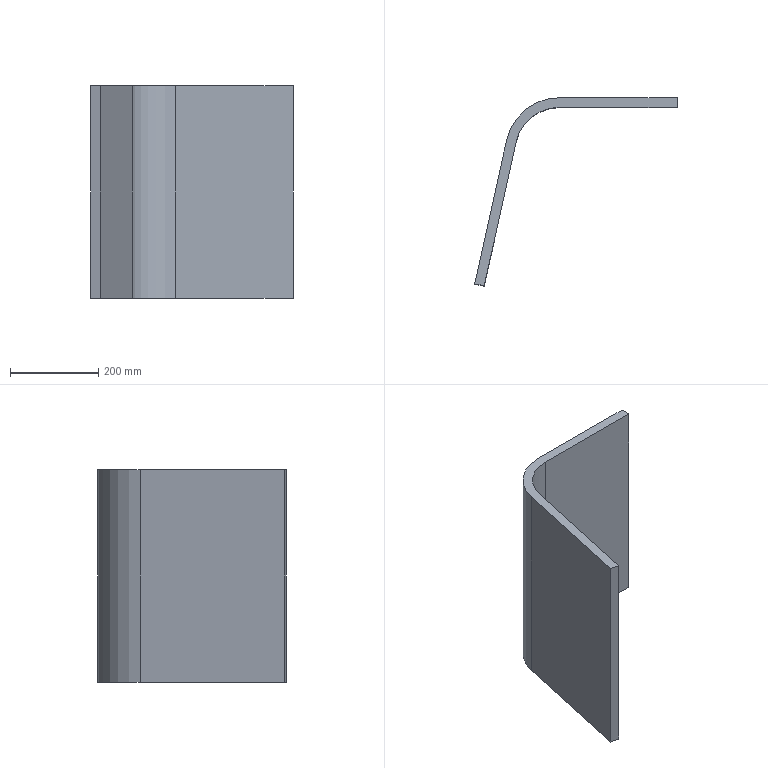Part | NX | features 底座(默认<按焊接>) 2 | 1 solid | 10 faces | box 457.703 x 425.5 x 480 mm | volume 7854055 mm3 | plane 8 | cylinder 2 | commonest cylinder face diameters 200 x1 243.64 x1
STEP:
#1=CARTESIAN_POINT('',(1554.365,567.32,-412.));
#2=VERTEX_POINT('',#1);
#3=CARTESIAN_POINT('',(1287.717,567.32,-412.));
#4=VERTEX_POINT('',#3);
#5=CARTESIAN_POINT('',(1250.85,567.32,-412.));
#6=DIRECTION('',(-1.,0.,0.));
#7=VECTOR('',#6,1000.);
#8=LINE('',#5,#7);
#9=EDGE_CURVE('',#2,#4,#8,.T.);
#10=ORIENTED_EDGE('',*,*,#9,.F.);
#11=CARTESIAN_POINT('',(1554.365,567.32,-892.));
#12=VERTEX_POINT('',#11);
#13=CARTESIAN_POINT('',(1554.365,567.32,-892.));
#14=DIRECTION('',(0.,0.,1.));
#15=VECTOR('',#14,1000.);
#16=LINE('',#13,#15);
#17=EDGE_CURVE('',#12,#2,#16,.T.);
#18=ORIENTED_EDGE('',*,*,#17,.F.);
#19=CARTESIAN_POINT('',(1287.717,567.32,-892.));
#20=VERTEX_POINT('',#19);
#21=CARTESIAN_POINT('',(1250.85,567.32,-892.));
#22=DIRECTION('',(-1.,0.,0.));
#23=VECTOR('',#22,1000.);
#24=LINE('',#21,#23);
#25=EDGE_CURVE('',#12,#20,#24,.T.);
#26=ORIENTED_EDGE('',*,*,#25,.T.);
#27=CARTESIAN_POINT('',(1287.717,567.32,-892.));
#28=DIRECTION('',(0.,0.,1.));
#29=VECTOR('',#28,1000.);
#30=LINE('',#27,#29);
#31=EDGE_CURVE('',#20,#4,#30,.T.);
#32=ORIENTED_EDGE('',*,*,#31,.T.);
#33=EDGE_LOOP('',(#10,#18,#26,#32));
#34=FACE_BOUND('',#33,.T.);
#35=CARTESIAN_POINT('',(1250.85,567.32,-892.));
#36=DIRECTION('',(0.,-1.,0.));
#37=DIRECTION('',(0.,0.,1.));
#38=AXIS2_PLACEMENT_3D('',#35,#36,#37);
#39=PLANE('',#38);
#40=ADVANCED_FACE('',(#34),#39,.F.);
#41=CARTESIAN_POINT('',(1168.785,471.867,-412.));
#42=VERTEX_POINT('',#41);
#43=CARTESIAN_POINT('',(1287.717,445.5,-412.));
#44=DIRECTION('',(0.,0.,1.));
#45=DIRECTION('',(1.,0.,0.));
#46=AXIS2_PLACEMENT_3D('',#43,#44,#45);
#47=CIRCLE('',#46,121.82);
#48=EDGE_CURVE('',#4,#42,#47,.T.);
#49=ORIENTED_EDGE('',*,*,#48,.F.);
#50=ORIENTED_EDGE('',*,*,#31,.F.);
#51=CARTESIAN_POINT('',(1168.785,471.867,-892.));
#52=VERTEX_POINT('',#51);
#53=CARTESIAN_POINT('',(1287.717,445.5,-892.));
#54=DIRECTION('',(0.,0.,1.));
#55=DIRECTION('',(1.,0.,0.));
#56=AXIS2_PLACEMENT_3D('',#53,#54,#55);
#57=CIRCLE('',#56,121.82);
#58=EDGE_CURVE('',#20,#52,#57,.T.);
#59=ORIENTED_EDGE('',*,*,#58,.T.);
#60=CARTESIAN_POINT('',(1168.785,471.867,-892.));
#61=DIRECTION('',(0.,0.,1.));
#62=VECTOR('',#61,1000.);
#63=LINE('',#60,#62);
#64=EDGE_CURVE('',#52,#42,#63,.T.);
#65=ORIENTED_EDGE('',*,*,#64,.T.);
#66=EDGE_LOOP('',(#49,#50,#59,#65));
#67=FACE_BOUND('',#66,.T.);
#68=CARTESIAN_POINT('',(1287.717,445.5,-892.));
#69=DIRECTION('',(0.,0.,1.));
#70=DIRECTION('',(-1.,0.,0.));
#71=AXIS2_PLACEMENT_3D('',#68,#69,#70);
#72=CYLINDRICAL_SURFACE('',#71,121.82);
#73=ADVANCED_FACE('',(#67),#72,.T.);
#74=CARTESIAN_POINT('',(1096.662,146.543,-412.));
#75=VERTEX_POINT('',#74);
#76=CARTESIAN_POINT('',(571.37,-2222.899,-412.));
#77=DIRECTION('',(0.2164,0.9763,0.));
#78=VECTOR('',#77,1000.);
#79=LINE('',#76,#78);
#80=EDGE_CURVE('',#75,#42,#79,.T.);
#81=ORIENTED_EDGE('',*,*,#80,.T.);
#82=ORIENTED_EDGE('',*,*,#64,.F.);
#83=CARTESIAN_POINT('',(1096.662,146.543,-892.));
#84=VERTEX_POINT('',#83);
#85=CARTESIAN_POINT('',(571.37,-2222.899,-892.));
#86=DIRECTION('',(0.2164,0.9763,0.));
#87=VECTOR('',#86,1000.);
#88=LINE('',#85,#87);
#89=EDGE_CURVE('',#84,#52,#88,.T.);
#90=ORIENTED_EDGE('',*,*,#89,.F.);
#91=CARTESIAN_POINT('',(1096.662,146.543,-892.));
#92=DIRECTION('',(0.,0.,1.));
#93=VECTOR('',#92,1000.);
#94=LINE('',#91,#93);
#95=EDGE_CURVE('',#84,#75,#94,.T.);
#96=ORIENTED_EDGE('',*,*,#95,.T.);
#97=EDGE_LOOP('',(#81,#82,#90,#96));
#98=FACE_BOUND('',#97,.T.);
#99=CARTESIAN_POINT('',(571.37,-2222.899,-892.));
#100=DIRECTION('',(-0.9763,0.2164,0.));
#101=DIRECTION('',(-0.2164,-0.9763,0.));
#102=AXIS2_PLACEMENT_3D('',#99,#100,#101);
#103=PLANE('',#102);
#104=ADVANCED_FACE('',(#98),#103,.T.);
#105=CARTESIAN_POINT('',(1117.965,141.82,-412.));
#106=VERTEX_POINT('',#105);
#107=CARTESIAN_POINT('',(1776.142,-4.094,-412.));
#108=DIRECTION('',(0.9763,-0.2164,0.));
#109=VECTOR('',#108,1000.);
#110=LINE('',#107,#109);
#111=EDGE_CURVE('',#75,#106,#110,.T.);
#112=ORIENTED_EDGE('',*,*,#111,.F.);
#113=ORIENTED_EDGE('',*,*,#95,.F.);
#114=CARTESIAN_POINT('',(1117.965,141.82,-892.));
#115=VERTEX_POINT('',#114);
#116=CARTESIAN_POINT('',(1776.142,-4.094,-892.));
#117=DIRECTION('',(0.9763,-0.2164,0.));
#118=VECTOR('',#117,1000.);
#119=LINE('',#116,#118);
#120=EDGE_CURVE('',#84,#115,#119,.T.);
#121=ORIENTED_EDGE('',*,*,#120,.T.);
#122=CARTESIAN_POINT('',(1117.965,141.82,-892.));
#123=DIRECTION('',(0.,0.,1.));
#124=VECTOR('',#123,1000.);
#125=LINE('',#122,#124);
#126=EDGE_CURVE('',#115,#106,#125,.T.);
#127=ORIENTED_EDGE('',*,*,#126,.T.);
#128=EDGE_LOOP('',(#112,#113,#121,#127));
#129=FACE_BOUND('',#128,.T.);
#130=CARTESIAN_POINT('',(1776.142,-4.094,-892.));
#131=DIRECTION('',(0.2164,0.9763,0.));
#132=DIRECTION('',(-0.9763,0.2164,0.));
#133=AXIS2_PLACEMENT_3D('',#130,#131,#132);
#134=PLANE('',#133);
#135=ADVANCED_FACE('',(#129),#134,.F.);
#136=CARTESIAN_POINT('',(1190.088,467.144,-412.));
#137=VERTEX_POINT('',#136);
#138=CARTESIAN_POINT('',(592.673,-2227.621,-412.));
#139=DIRECTION('',(0.2164,0.9763,0.));
#140=VECTOR('',#139,1000.);
#141=LINE('',#138,#140);
#142=EDGE_CURVE('',#106,#137,#141,.T.);
#143=ORIENTED_EDGE('',*,*,#142,.F.);
#144=ORIENTED_EDGE('',*,*,#126,.F.);
#145=CARTESIAN_POINT('',(1190.088,467.144,-892.));
#146=VERTEX_POINT('',#145);
#147=CARTESIAN_POINT('',(592.673,-2227.621,-892.));
#148=DIRECTION('',(0.2164,0.9763,0.));
#149=VECTOR('',#148,1000.);
#150=LINE('',#147,#149);
#151=EDGE_CURVE('',#115,#146,#150,.T.);
#152=ORIENTED_EDGE('',*,*,#151,.T.);
#153=CARTESIAN_POINT('',(1190.088,467.144,-892.));
#154=DIRECTION('',(0.,0.,1.));
#155=VECTOR('',#154,1000.);
#156=LINE('',#153,#155);
#157=EDGE_CURVE('',#146,#137,#156,.T.);
#158=ORIENTED_EDGE('',*,*,#157,.T.);
#159=EDGE_LOOP('',(#143,#144,#152,#158));
#160=FACE_BOUND('',#159,.T.);
#161=CARTESIAN_POINT('',(592.673,-2227.621,-892.));
#162=DIRECTION('',(-0.9763,0.2164,0.));
#163=DIRECTION('',(-0.2164,-0.9763,0.));
#164=AXIS2_PLACEMENT_3D('',#161,#162,#163);
#165=PLANE('',#164);
#166=ADVANCED_FACE('',(#160),#165,.F.);
#167=CARTESIAN_POINT('',(1287.717,545.5,-412.));
#168=VERTEX_POINT('',#167);
#169=CARTESIAN_POINT('',(1287.717,445.5,-412.));
#170=DIRECTION('',(0.,0.,1.));
#171=DIRECTION('',(1.,0.,0.));
#172=AXIS2_PLACEMENT_3D('',#169,#170,#171);
#173=CIRCLE('',#172,100.);
#174=EDGE_CURVE('',#168,#137,#173,.T.);
#175=ORIENTED_EDGE('',*,*,#174,.T.);
#176=ORIENTED_EDGE('',*,*,#157,.F.);
#177=CARTESIAN_POINT('',(1287.717,545.5,-892.));
#178=VERTEX_POINT('',#177);
#179=CARTESIAN_POINT('',(1287.717,445.5,-892.));
#180=DIRECTION('',(0.,0.,1.));
#181=DIRECTION('',(1.,0.,0.));
#182=AXIS2_PLACEMENT_3D('',#179,#180,#181);
#183=CIRCLE('',#182,100.);
#184=EDGE_CURVE('',#178,#146,#183,.T.);
#185=ORIENTED_EDGE('',*,*,#184,.F.);
#186=CARTESIAN_POINT('',(1287.717,545.5,-892.));
#187=DIRECTION('',(0.,0.,1.));
#188=VECTOR('',#187,1000.);
#189=LINE('',#186,#188);
#190=EDGE_CURVE('',#178,#168,#189,.T.);
#191=ORIENTED_EDGE('',*,*,#190,.T.);
#192=EDGE_LOOP('',(#175,#176,#185,#191));
#193=FACE_BOUND('',#192,.T.);
#194=CARTESIAN_POINT('',(1287.717,445.5,-892.));
#195=DIRECTION('',(0.,0.,1.));
#196=DIRECTION('',(-1.,0.,0.));
#197=AXIS2_PLACEMENT_3D('',#194,#195,#196);
#198=CYLINDRICAL_SURFACE('',#197,100.);
#199=ADVANCED_FACE('',(#193),#198,.F.);
#200=CARTESIAN_POINT('',(1554.365,545.5,-412.));
#201=VERTEX_POINT('',#200);
#202=CARTESIAN_POINT('',(1250.85,545.5,-412.));
#203=DIRECTION('',(-1.,0.,0.));
#204=VECTOR('',#203,1000.);
#205=LINE('',#202,#204);
#206=EDGE_CURVE('',#201,#168,#205,.T.);
#207=ORIENTED_EDGE('',*,*,#206,.T.);
#208=ORIENTED_EDGE('',*,*,#190,.F.);
#209=CARTESIAN_POINT('',(1554.365,545.5,-892.));
#210=VERTEX_POINT('',#209);
#211=CARTESIAN_POINT('',(1250.85,545.5,-892.));
#212=DIRECTION('',(-1.,0.,0.));
#213=VECTOR('',#212,1000.);
#214=LINE('',#211,#213);
#215=EDGE_CURVE('',#210,#178,#214,.T.);
#216=ORIENTED_EDGE('',*,*,#215,.F.);
#217=CARTESIAN_POINT('',(1554.365,545.5,-892.));
#218=DIRECTION('',(0.,0.,1.));
#219=VECTOR('',#218,1000.);
#220=LINE('',#217,#219);
#221=EDGE_CURVE('',#210,#201,#220,.T.);
#222=ORIENTED_EDGE('',*,*,#221,.T.);
#223=EDGE_LOOP('',(#207,#208,#216,#222));
#224=FACE_BOUND('',#223,.T.);
#225=CARTESIAN_POINT('',(1250.85,545.5,-892.));
#226=DIRECTION('',(0.,-1.,0.));
#227=DIRECTION('',(0.,0.,1.));
#228=AXIS2_PLACEMENT_3D('',#225,#226,#227);
#229=PLANE('',#228);
#230=ADVANCED_FACE('',(#224),#229,.T.);
#231=CARTESIAN_POINT('',(1554.365,-2373.536,-412.));
#232=DIRECTION('',(0.,-1.,0.));
#233=VECTOR('',#232,1000.);
#234=LINE('',#231,#233);
#235=EDGE_CURVE('',#2,#201,#234,.T.);
#236=ORIENTED_EDGE('',*,*,#235,.T.);
#237=ORIENTED_EDGE('',*,*,#221,.F.);
#238=CARTESIAN_POINT('',(1554.365,-2373.536,-892.));
#239=DIRECTION('',(0.,-1.,0.));
#240=VECTOR('',#239,1000.);
#241=LINE('',#238,#240);
#242=EDGE_CURVE('',#12,#210,#241,.T.);
#243=ORIENTED_EDGE('',*,*,#242,.F.);
#244=ORIENTED_EDGE('',*,*,#17,.T.);
#245=EDGE_LOOP('',(#236,#237,#243,#244));
#246=FACE_BOUND('',#245,.T.);
#247=CARTESIAN_POINT('',(1554.365,-2373.536,-892.));
#248=DIRECTION('',(1.,0.,0.));
#249=DIRECTION('',(0.,0.,1.));
#250=AXIS2_PLACEMENT_3D('',#247,#248,#249);
#251=PLANE('',#250);
#252=ADVANCED_FACE('',(#246),#251,.T.);
#253=ORIENTED_EDGE('',*,*,#25,.F.);
#254=ORIENTED_EDGE('',*,*,#242,.T.);
#255=ORIENTED_EDGE('',*,*,#215,.T.);
#256=ORIENTED_EDGE('',*,*,#184,.T.);
#257=ORIENTED_EDGE('',*,*,#151,.F.);
#258=ORIENTED_EDGE('',*,*,#120,.F.);
#259=ORIENTED_EDGE('',*,*,#89,.T.);
#260=ORIENTED_EDGE('',*,*,#58,.F.);
#261=EDGE_LOOP('',(#253,#254,#255,#256,#257,#258,#259,#260));
#262=FACE_BOUND('',#261,.T.);
#263=CARTESIAN_POINT('',(1250.85,-2373.536,-892.));
#264=DIRECTION('',(0.,0.,-1.));
#265=DIRECTION('',(1.,0.,0.));
#266=AXIS2_PLACEMENT_3D('',#263,#264,#265);
#267=PLANE('',#266);
#268=ADVANCED_FACE('',(#262),#267,.T.);
#269=ORIENTED_EDGE('',*,*,#9,.T.);
#270=ORIENTED_EDGE('',*,*,#48,.T.);
#271=ORIENTED_EDGE('',*,*,#80,.F.);
#272=ORIENTED_EDGE('',*,*,#111,.T.);
#273=ORIENTED_EDGE('',*,*,#142,.T.);
#274=ORIENTED_EDGE('',*,*,#174,.F.);
#275=ORIENTED_EDGE('',*,*,#206,.F.);
#276=ORIENTED_EDGE('',*,*,#235,.F.);
#277=EDGE_LOOP('',(#269,#270,#271,#272,#273,#274,#275,#276));
#278=FACE_BOUND('',#277,.T.);
#279=CARTESIAN_POINT('',(1250.85,-2373.536,-412.));
#280=DIRECTION('',(0.,0.,-1.));
#281=DIRECTION('',(1.,0.,0.));
#282=AXIS2_PLACEMENT_3D('',#279,#280,#281);
#283=PLANE('',#282);
#284=ADVANCED_FACE('',(#278),#283,.F.);
#285=CLOSED_SHELL('',(#40,#73,#104,#135,#166,#199,#230,#252,#268,#284));
#286=MANIFOLD_SOLID_BREP('',#285);
#287=(LENGTH_UNIT()NAMED_UNIT(*)SI_UNIT(.MILLI.,.METRE.));
#288=UNCERTAINTY_MEASURE_WITH_UNIT(LENGTH_MEASURE(0.00001),#287,'','');
#289=(NAMED_UNIT(*)PLANE_ANGLE_UNIT()SI_UNIT($,.RADIAN.));
#290=(NAMED_UNIT(*)SI_UNIT($,.STERADIAN.)SOLID_ANGLE_UNIT());
#291=(GEOMETRIC_REPRESENTATION_CONTEXT(3)GLOBAL_UNCERTAINTY_ASSIGNED_CONTEXT((#288))GLOBAL_UNIT_ASSIGNED_CONTEXT((#287,#289,#290))REPRESENTATION_CONTEXT('',''));
#292=ADVANCED_BREP_SHAPE_REPRESENTATION('',(#286),#291);